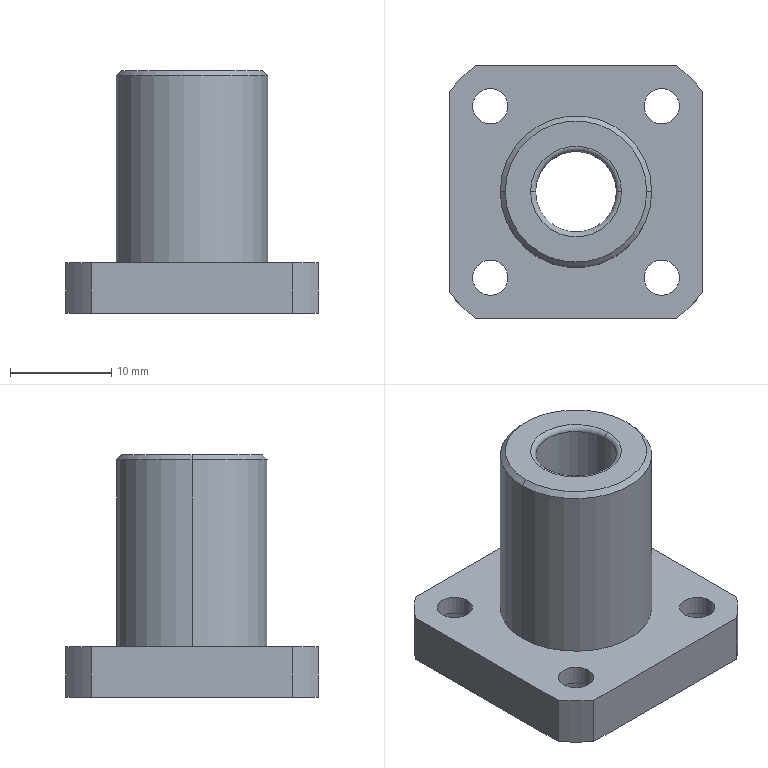Part | STEP file | linear bearing LMK8UU_Default | 1 solid | 41 faces | box 25 x 25 x 24 mm | volume 4786 mm3 | cylinder 24 | plane 11 | torus 4 | cone 2 | commonest cylinder face diameters 3.5 x8 6 x8 32 x4 8 x2 15 x2